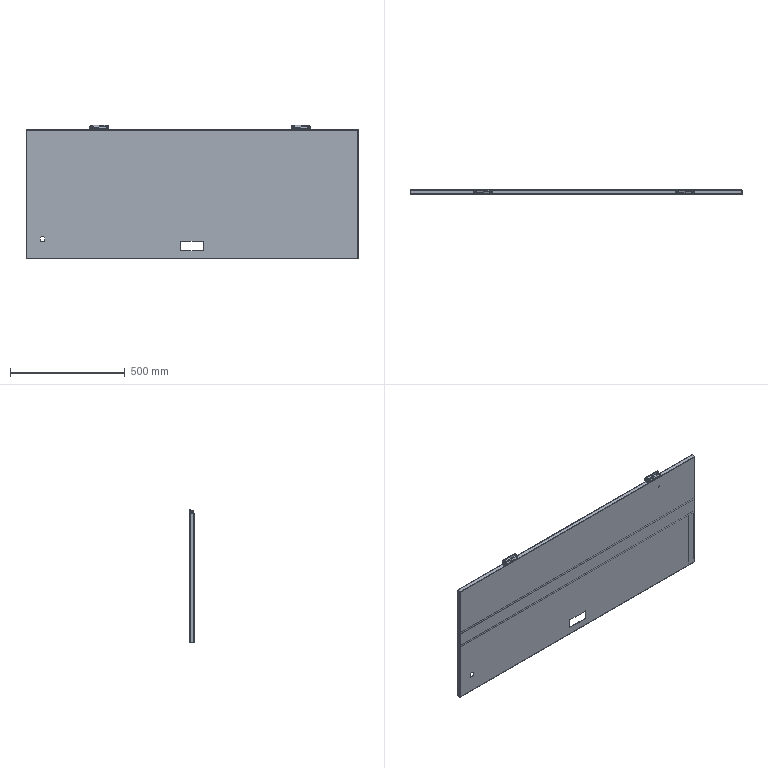Part | SolidWorks | 7 solids | 293 faces | box 1445 x 20.5 x 580.25 mm | volume 1660730 mm3 | plane 165 | cylinder 104 | cone 16 | spline 8 | commonest cylinder face diameters 0.4 x16 3.3 x16 3.4 x16 4.2 x16 8 x14 14.5 x12